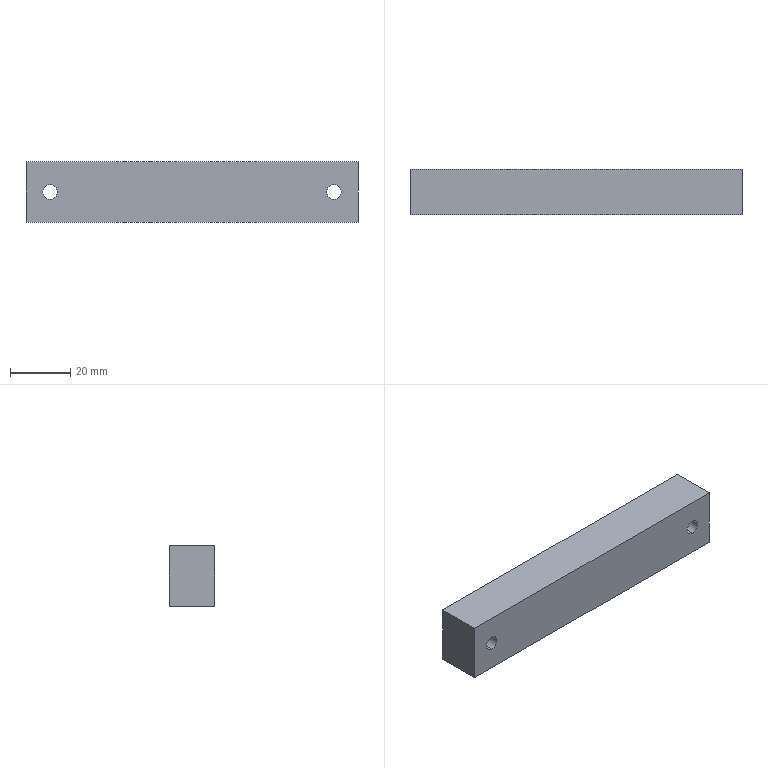Part | SolidWorks | features Extrusion 1, HoleWzd 1 | 1 solid | 10 faces | box 110 x 15 x 20 mm | volume 32457 mm3 | plane 6 | cylinder 4 | commonest cylinder face diameters 4.8 x4
STEP:
#1=CARTESIAN_POINT('',(-47.,0.,-2.4));
#2=VERTEX_POINT('',#1);
#3=CARTESIAN_POINT('',(-47.,0.,2.4));
#4=VERTEX_POINT('',#3);
#5=CARTESIAN_POINT('',(-47.,0.,0.));
#6=DIRECTION('',(0.,1.,0.));
#7=DIRECTION('',(0.,0.,1.));
#8=AXIS2_PLACEMENT_3D('',#5,#6,#7);
#9=CIRCLE('',#8,2.4);
#10=EDGE_CURVE('',#2,#4,#9,.T.);
#11=ORIENTED_EDGE('',*,*,#10,.F.);
#12=CARTESIAN_POINT('',(-47.,15.,-2.4));
#13=VERTEX_POINT('',#12);
#14=CARTESIAN_POINT('',(-47.,15.,-2.4));
#15=DIRECTION('',(0.,1.,0.));
#16=VECTOR('',#15,1000.);
#17=LINE('',#14,#16);
#18=EDGE_CURVE('',#2,#13,#17,.T.);
#19=ORIENTED_EDGE('',*,*,#18,.T.);
#20=CARTESIAN_POINT('',(-47.,15.,2.4));
#21=VERTEX_POINT('',#20);
#22=CARTESIAN_POINT('',(-47.,15.,0.));
#23=DIRECTION('',(0.,1.,0.));
#24=DIRECTION('',(0.,0.,1.));
#25=AXIS2_PLACEMENT_3D('',#22,#23,#24);
#26=CIRCLE('',#25,2.4);
#27=EDGE_CURVE('',#13,#21,#26,.T.);
#28=ORIENTED_EDGE('',*,*,#27,.T.);
#29=CARTESIAN_POINT('',(-47.,15.,2.4));
#30=DIRECTION('',(0.,1.,0.));
#31=VECTOR('',#30,1000.);
#32=LINE('',#29,#31);
#33=EDGE_CURVE('',#4,#21,#32,.T.);
#34=ORIENTED_EDGE('',*,*,#33,.F.);
#35=EDGE_LOOP('',(#11,#19,#28,#34));
#36=FACE_OUTER_BOUND('',#35,.T.);
#37=CARTESIAN_POINT('',(-47.,15.,0.));
#38=DIRECTION('',(0.,1.,0.));
#39=DIRECTION('',(0.,0.,1.));
#40=AXIS2_PLACEMENT_3D('',#37,#38,#39);
#41=CYLINDRICAL_SURFACE('',#40,2.4);
#42=ADVANCED_FACE('',(#36),#41,.F.);
#43=CARTESIAN_POINT('',(47.,0.,-2.4));
#44=VERTEX_POINT('',#43);
#45=CARTESIAN_POINT('',(47.,0.,2.4));
#46=VERTEX_POINT('',#45);
#47=CARTESIAN_POINT('',(47.,0.,0.));
#48=DIRECTION('',(0.,1.,0.));
#49=DIRECTION('',(0.,0.,1.));
#50=AXIS2_PLACEMENT_3D('',#47,#48,#49);
#51=CIRCLE('',#50,2.4);
#52=EDGE_CURVE('',#44,#46,#51,.T.);
#53=ORIENTED_EDGE('',*,*,#52,.F.);
#54=CARTESIAN_POINT('',(47.,15.,-2.4));
#55=VERTEX_POINT('',#54);
#56=CARTESIAN_POINT('',(47.,15.,-2.4));
#57=DIRECTION('',(0.,1.,0.));
#58=VECTOR('',#57,1000.);
#59=LINE('',#56,#58);
#60=EDGE_CURVE('',#44,#55,#59,.T.);
#61=ORIENTED_EDGE('',*,*,#60,.T.);
#62=CARTESIAN_POINT('',(47.,15.,2.4));
#63=VERTEX_POINT('',#62);
#64=CARTESIAN_POINT('',(47.,15.,0.));
#65=DIRECTION('',(0.,1.,0.));
#66=DIRECTION('',(0.,0.,1.));
#67=AXIS2_PLACEMENT_3D('',#64,#65,#66);
#68=CIRCLE('',#67,2.4);
#69=EDGE_CURVE('',#55,#63,#68,.T.);
#70=ORIENTED_EDGE('',*,*,#69,.T.);
#71=CARTESIAN_POINT('',(47.,15.,2.4));
#72=DIRECTION('',(0.,1.,0.));
#73=VECTOR('',#72,1000.);
#74=LINE('',#71,#73);
#75=EDGE_CURVE('',#46,#63,#74,.T.);
#76=ORIENTED_EDGE('',*,*,#75,.F.);
#77=EDGE_LOOP('',(#53,#61,#70,#76));
#78=FACE_OUTER_BOUND('',#77,.T.);
#79=CARTESIAN_POINT('',(47.,15.,0.));
#80=DIRECTION('',(0.,1.,0.));
#81=DIRECTION('',(0.,0.,1.));
#82=AXIS2_PLACEMENT_3D('',#79,#80,#81);
#83=CYLINDRICAL_SURFACE('',#82,2.4);
#84=ADVANCED_FACE('',(#78),#83,.F.);
#85=CARTESIAN_POINT('',(55.,0.,10.));
#86=VERTEX_POINT('',#85);
#87=CARTESIAN_POINT('',(55.,0.,-10.));
#88=VERTEX_POINT('',#87);
#89=CARTESIAN_POINT('',(55.,0.,10.));
#90=DIRECTION('',(0.,0.,-1.));
#91=VECTOR('',#90,1000.);
#92=LINE('',#89,#91);
#93=EDGE_CURVE('',#86,#88,#92,.T.);
#94=ORIENTED_EDGE('',*,*,#93,.T.);
#95=CARTESIAN_POINT('',(55.,15.,-10.));
#96=VERTEX_POINT('',#95);
#97=CARTESIAN_POINT('',(55.,15.,-10.));
#98=DIRECTION('',(0.,-1.,0.));
#99=VECTOR('',#98,1000.);
#100=LINE('',#97,#99);
#101=EDGE_CURVE('',#96,#88,#100,.T.);
#102=ORIENTED_EDGE('',*,*,#101,.F.);
#103=CARTESIAN_POINT('',(55.,15.,10.));
#104=VERTEX_POINT('',#103);
#105=CARTESIAN_POINT('',(55.,15.,10.));
#106=DIRECTION('',(0.,0.,-1.));
#107=VECTOR('',#106,1000.);
#108=LINE('',#105,#107);
#109=EDGE_CURVE('',#104,#96,#108,.T.);
#110=ORIENTED_EDGE('',*,*,#109,.F.);
#111=CARTESIAN_POINT('',(55.,15.,10.));
#112=DIRECTION('',(0.,-1.,0.));
#113=VECTOR('',#112,1000.);
#114=LINE('',#111,#113);
#115=EDGE_CURVE('',#104,#86,#114,.T.);
#116=ORIENTED_EDGE('',*,*,#115,.T.);
#117=EDGE_LOOP('',(#94,#102,#110,#116));
#118=FACE_OUTER_BOUND('',#117,.T.);
#119=CARTESIAN_POINT('',(55.,15.,10.));
#120=DIRECTION('',(-1.,0.,0.));
#121=DIRECTION('',(0.,0.,1.));
#122=AXIS2_PLACEMENT_3D('',#119,#120,#121);
#123=PLANE('',#122);
#124=ADVANCED_FACE('',(#118),#123,.F.);
#125=CARTESIAN_POINT('',(-55.,0.,-10.));
#126=VERTEX_POINT('',#125);
#127=CARTESIAN_POINT('',(-55.,0.,-10.));
#128=DIRECTION('',(-1.,0.,0.));
#129=VECTOR('',#128,1000.);
#130=LINE('',#127,#129);
#131=EDGE_CURVE('',#88,#126,#130,.T.);
#132=ORIENTED_EDGE('',*,*,#131,.T.);
#133=CARTESIAN_POINT('',(-55.,15.,-10.));
#134=VERTEX_POINT('',#133);
#135=CARTESIAN_POINT('',(-55.,15.,-10.));
#136=DIRECTION('',(0.,-1.,0.));
#137=VECTOR('',#136,1000.);
#138=LINE('',#135,#137);
#139=EDGE_CURVE('',#134,#126,#138,.T.);
#140=ORIENTED_EDGE('',*,*,#139,.F.);
#141=CARTESIAN_POINT('',(-55.,15.,-10.));
#142=DIRECTION('',(-1.,0.,0.));
#143=VECTOR('',#142,1000.);
#144=LINE('',#141,#143);
#145=EDGE_CURVE('',#96,#134,#144,.T.);
#146=ORIENTED_EDGE('',*,*,#145,.F.);
#147=ORIENTED_EDGE('',*,*,#101,.T.);
#148=EDGE_LOOP('',(#132,#140,#146,#147));
#149=FACE_OUTER_BOUND('',#148,.T.);
#150=CARTESIAN_POINT('',(-55.,15.,-10.));
#151=DIRECTION('',(0.,0.,1.));
#152=DIRECTION('',(1.,0.,0.));
#153=AXIS2_PLACEMENT_3D('',#150,#151,#152);
#154=PLANE('',#153);
#155=ADVANCED_FACE('',(#149),#154,.F.);
#156=CARTESIAN_POINT('',(-55.,0.,10.));
#157=VERTEX_POINT('',#156);
#158=CARTESIAN_POINT('',(-55.,0.,10.));
#159=DIRECTION('',(0.,0.,1.));
#160=VECTOR('',#159,1000.);
#161=LINE('',#158,#160);
#162=EDGE_CURVE('',#126,#157,#161,.T.);
#163=ORIENTED_EDGE('',*,*,#162,.T.);
#164=CARTESIAN_POINT('',(-55.,15.,10.));
#165=VERTEX_POINT('',#164);
#166=CARTESIAN_POINT('',(-55.,15.,10.));
#167=DIRECTION('',(0.,-1.,0.));
#168=VECTOR('',#167,1000.);
#169=LINE('',#166,#168);
#170=EDGE_CURVE('',#165,#157,#169,.T.);
#171=ORIENTED_EDGE('',*,*,#170,.F.);
#172=CARTESIAN_POINT('',(-55.,15.,10.));
#173=DIRECTION('',(0.,0.,1.));
#174=VECTOR('',#173,1000.);
#175=LINE('',#172,#174);
#176=EDGE_CURVE('',#134,#165,#175,.T.);
#177=ORIENTED_EDGE('',*,*,#176,.F.);
#178=ORIENTED_EDGE('',*,*,#139,.T.);
#179=EDGE_LOOP('',(#163,#171,#177,#178));
#180=FACE_OUTER_BOUND('',#179,.T.);
#181=CARTESIAN_POINT('',(-55.,15.,10.));
#182=DIRECTION('',(1.,0.,0.));
#183=DIRECTION('',(0.,0.,-1.));
#184=AXIS2_PLACEMENT_3D('',#181,#182,#183);
#185=PLANE('',#184);
#186=ADVANCED_FACE('',(#180),#185,.F.);
#187=CARTESIAN_POINT('',(-55.,0.,10.));
#188=DIRECTION('',(1.,0.,0.));
#189=VECTOR('',#188,1000.);
#190=LINE('',#187,#189);
#191=EDGE_CURVE('',#157,#86,#190,.T.);
#192=ORIENTED_EDGE('',*,*,#191,.T.);
#193=ORIENTED_EDGE('',*,*,#115,.F.);
#194=CARTESIAN_POINT('',(-55.,15.,10.));
#195=DIRECTION('',(1.,0.,0.));
#196=VECTOR('',#195,1000.);
#197=LINE('',#194,#196);
#198=EDGE_CURVE('',#165,#104,#197,.T.);
#199=ORIENTED_EDGE('',*,*,#198,.F.);
#200=ORIENTED_EDGE('',*,*,#170,.T.);
#201=EDGE_LOOP('',(#192,#193,#199,#200));
#202=FACE_OUTER_BOUND('',#201,.T.);
#203=CARTESIAN_POINT('',(-55.,15.,10.));
#204=DIRECTION('',(0.,0.,-1.));
#205=DIRECTION('',(-1.,0.,0.));
#206=AXIS2_PLACEMENT_3D('',#203,#204,#205);
#207=PLANE('',#206);
#208=ADVANCED_FACE('',(#202),#207,.F.);
#209=CARTESIAN_POINT('',(-47.,15.,0.));
#210=DIRECTION('',(0.,1.,0.));
#211=DIRECTION('',(0.,0.,1.));
#212=AXIS2_PLACEMENT_3D('',#209,#210,#211);
#213=CIRCLE('',#212,2.4);
#214=EDGE_CURVE('',#21,#13,#213,.T.);
#215=ORIENTED_EDGE('',*,*,#214,.F.);
#216=ORIENTED_EDGE('',*,*,#27,.F.);
#217=EDGE_LOOP('',(#215,#216));
#218=FACE_BOUND('',#217,.T.);
#219=CARTESIAN_POINT('',(47.,15.,0.));
#220=DIRECTION('',(0.,1.,0.));
#221=DIRECTION('',(0.,0.,1.));
#222=AXIS2_PLACEMENT_3D('',#219,#220,#221);
#223=CIRCLE('',#222,2.4);
#224=EDGE_CURVE('',#63,#55,#223,.T.);
#225=ORIENTED_EDGE('',*,*,#224,.F.);
#226=ORIENTED_EDGE('',*,*,#69,.F.);
#227=EDGE_LOOP('',(#225,#226));
#228=FACE_BOUND('',#227,.T.);
#229=ORIENTED_EDGE('',*,*,#109,.T.);
#230=ORIENTED_EDGE('',*,*,#145,.T.);
#231=ORIENTED_EDGE('',*,*,#176,.T.);
#232=ORIENTED_EDGE('',*,*,#198,.T.);
#233=EDGE_LOOP('',(#229,#230,#231,#232));
#234=FACE_OUTER_BOUND('',#233,.T.);
#235=CARTESIAN_POINT('',(0.,15.,0.));
#236=DIRECTION('',(0.,-1.,0.));
#237=DIRECTION('',(0.,0.,-1.));
#238=AXIS2_PLACEMENT_3D('',#235,#236,#237);
#239=PLANE('',#238);
#240=ADVANCED_FACE('',(#218,#228,#234),#239,.F.);
#241=CARTESIAN_POINT('',(-47.,0.,0.));
#242=DIRECTION('',(0.,1.,0.));
#243=DIRECTION('',(0.,0.,1.));
#244=AXIS2_PLACEMENT_3D('',#241,#242,#243);
#245=CIRCLE('',#244,2.4);
#246=EDGE_CURVE('',#4,#2,#245,.T.);
#247=ORIENTED_EDGE('',*,*,#246,.T.);
#248=ORIENTED_EDGE('',*,*,#10,.T.);
#249=EDGE_LOOP('',(#247,#248));
#250=FACE_BOUND('',#249,.T.);
#251=CARTESIAN_POINT('',(47.,0.,0.));
#252=DIRECTION('',(0.,1.,0.));
#253=DIRECTION('',(0.,0.,1.));
#254=AXIS2_PLACEMENT_3D('',#251,#252,#253);
#255=CIRCLE('',#254,2.4);
#256=EDGE_CURVE('',#46,#44,#255,.T.);
#257=ORIENTED_EDGE('',*,*,#256,.T.);
#258=ORIENTED_EDGE('',*,*,#52,.T.);
#259=EDGE_LOOP('',(#257,#258));
#260=FACE_BOUND('',#259,.T.);
#261=ORIENTED_EDGE('',*,*,#93,.F.);
#262=ORIENTED_EDGE('',*,*,#191,.F.);
#263=ORIENTED_EDGE('',*,*,#162,.F.);
#264=ORIENTED_EDGE('',*,*,#131,.F.);
#265=EDGE_LOOP('',(#261,#262,#263,#264));
#266=FACE_OUTER_BOUND('',#265,.T.);
#267=CARTESIAN_POINT('',(0.,0.,0.));
#268=DIRECTION('',(0.,-1.,0.));
#269=DIRECTION('',(0.,0.,-1.));
#270=AXIS2_PLACEMENT_3D('',#267,#268,#269);
#271=PLANE('',#270);
#272=ADVANCED_FACE('',(#250,#260,#266),#271,.T.);
#273=ORIENTED_EDGE('',*,*,#60,.F.);
#274=ORIENTED_EDGE('',*,*,#256,.F.);
#275=ORIENTED_EDGE('',*,*,#75,.T.);
#276=ORIENTED_EDGE('',*,*,#224,.T.);
#277=EDGE_LOOP('',(#273,#274,#275,#276));
#278=FACE_OUTER_BOUND('',#277,.T.);
#279=CARTESIAN_POINT('',(47.,15.,0.));
#280=DIRECTION('',(0.,1.,0.));
#281=DIRECTION('',(0.,0.,1.));
#282=AXIS2_PLACEMENT_3D('',#279,#280,#281);
#283=CYLINDRICAL_SURFACE('',#282,2.4);
#284=ADVANCED_FACE('',(#278),#283,.F.);
#285=ORIENTED_EDGE('',*,*,#18,.F.);
#286=ORIENTED_EDGE('',*,*,#246,.F.);
#287=ORIENTED_EDGE('',*,*,#33,.T.);
#288=ORIENTED_EDGE('',*,*,#214,.T.);
#289=EDGE_LOOP('',(#285,#286,#287,#288));
#290=FACE_OUTER_BOUND('',#289,.T.);
#291=CARTESIAN_POINT('',(-47.,15.,0.));
#292=DIRECTION('',(0.,1.,0.));
#293=DIRECTION('',(0.,0.,1.));
#294=AXIS2_PLACEMENT_3D('',#291,#292,#293);
#295=CYLINDRICAL_SURFACE('',#294,2.4);
#296=ADVANCED_FACE('',(#290),#295,.F.);
#297=CLOSED_SHELL('',(#42,#84,#124,#155,#186,#208,#240,#272,#284,#296));
#298=MANIFOLD_SOLID_BREP('',#297);
#299=CARTESIAN_POINT('',(0.,0.,0.));
#300=DIRECTION('',(0.,0.,1.));
#301=DIRECTION('',(1.,0.,0.));
#302=AXIS2_PLACEMENT_3D('',#299,#300,#301);
#303=(LENGTH_UNIT()NAMED_UNIT(*)SI_UNIT(.MILLI.,.METRE.));
#304=UNCERTAINTY_MEASURE_WITH_UNIT(LENGTH_MEASURE(0.00001),#303,'','');
#305=(NAMED_UNIT(*)PLANE_ANGLE_UNIT()SI_UNIT($,.RADIAN.));
#306=(NAMED_UNIT(*)SI_UNIT($,.STERADIAN.)SOLID_ANGLE_UNIT());
#307=(GEOMETRIC_REPRESENTATION_CONTEXT(3)GLOBAL_UNCERTAINTY_ASSIGNED_CONTEXT((#304))GLOBAL_UNIT_ASSIGNED_CONTEXT((#303,#305,#306))REPRESENTATION_CONTEXT('',''));
#308=ADVANCED_BREP_SHAPE_REPRESENTATION('',(#298,#302),#307);